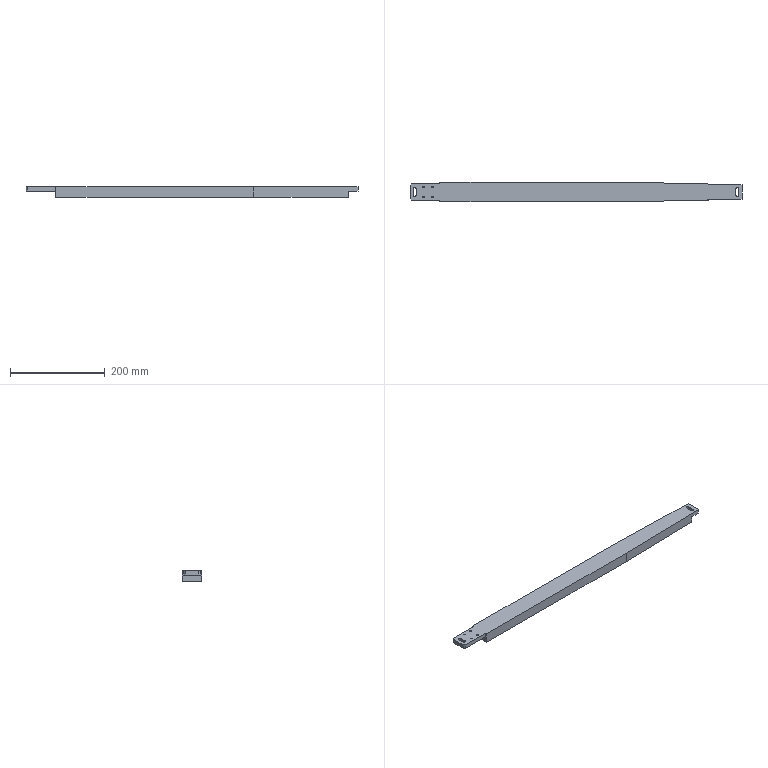Part | STEP file | PN_0003 | 1 solid | 32 faces | box 700 x 40.5 x 22 mm | volume 552490 mm3 | plane 20 | cylinder 12 | commonest cylinder face diameters 3.3 x8 6.5 x4